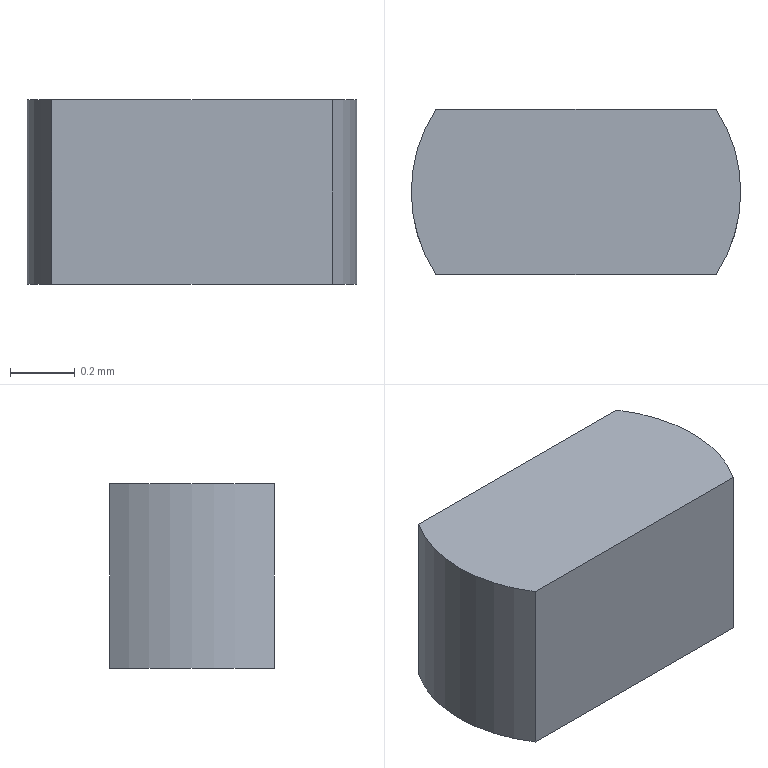Part | Creo | 1 solid | 6 faces | box 1.016 x 0.508 x 0.568 mm | volume 0.279 mm3 | plane 4 | cylinder 2 | commonest cylinder face diameters 0.923 x2
STEP:
#1=CARTESIAN_POINT('',(0.,0.,0.));
#2=DIRECTION('',(0.,0.,1.));
#3=DIRECTION('',(1.,0.,0.));
#4=AXIS2_PLACEMENT_3D('',#1,#2,#3);
#5=CARTESIAN_POINT('',(-0.4318,0.254,0.));
#6=VERTEX_POINT('',#5);
#7=CARTESIAN_POINT('',(-0.508,0.,0.));
#8=VERTEX_POINT('',#7);
#9=CARTESIAN_POINT('',(-0.04659,0.,0.));
#10=DIRECTION('',(0.,0.,1.));
#11=DIRECTION('',(-0.8348,0.5505,0.));
#12=AXIS2_PLACEMENT_3D('',#9,#10,#11);
#13=CIRCLE('',#12,0.4614);
#14=EDGE_CURVE('',#6,#8,#13,.T.);
#15=ORIENTED_EDGE('',*,*,#14,.T.);
#16=CARTESIAN_POINT('',(-0.4318,-0.254,0.));
#17=VERTEX_POINT('',#16);
#18=CARTESIAN_POINT('',(-0.04659,0.,0.));
#19=DIRECTION('',(0.,0.,1.));
#20=DIRECTION('',(-1.,0.,0.));
#21=AXIS2_PLACEMENT_3D('',#18,#19,#20);
#22=CIRCLE('',#21,0.4614);
#23=EDGE_CURVE('',#8,#17,#22,.T.);
#24=ORIENTED_EDGE('',*,*,#23,.T.);
#25=CARTESIAN_POINT('',(0.4318,-0.254,0.));
#26=VERTEX_POINT('',#25);
#27=CARTESIAN_POINT('',(-0.4318,-0.254,0.));
#28=DIRECTION('',(1.,0.,0.));
#29=VECTOR('',#28,0.8636);
#30=LINE('',#27,#29);
#31=EDGE_CURVE('',#17,#26,#30,.T.);
#32=ORIENTED_EDGE('',*,*,#31,.T.);
#33=CARTESIAN_POINT('',(0.508,0.,0.));
#34=VERTEX_POINT('',#33);
#35=CARTESIAN_POINT('',(0.04659,0.,0.));
#36=DIRECTION('',(0.,0.,1.));
#37=DIRECTION('',(0.8348,-0.5505,0.));
#38=AXIS2_PLACEMENT_3D('',#35,#36,#37);
#39=CIRCLE('',#38,0.4614);
#40=EDGE_CURVE('',#26,#34,#39,.T.);
#41=ORIENTED_EDGE('',*,*,#40,.T.);
#42=CARTESIAN_POINT('',(0.4318,0.254,0.));
#43=VERTEX_POINT('',#42);
#44=CARTESIAN_POINT('',(0.04659,0.,0.));
#45=DIRECTION('',(0.,0.,1.));
#46=DIRECTION('',(1.,0.,0.));
#47=AXIS2_PLACEMENT_3D('',#44,#45,#46);
#48=CIRCLE('',#47,0.4614);
#49=EDGE_CURVE('',#34,#43,#48,.T.);
#50=ORIENTED_EDGE('',*,*,#49,.T.);
#51=CARTESIAN_POINT('',(0.4318,0.254,0.));
#52=DIRECTION('',(-1.,0.,0.));
#53=VECTOR('',#52,0.8636);
#54=LINE('',#51,#53);
#55=EDGE_CURVE('',#43,#6,#54,.T.);
#56=ORIENTED_EDGE('',*,*,#55,.T.);
#57=EDGE_LOOP('',(#15,#24,#32,#41,#50,#56));
#58=FACE_OUTER_BOUND('',#57,.F.);
#59=CARTESIAN_POINT('',(0.,0.,0.));
#60=DIRECTION('',(0.,0.,1.));
#61=DIRECTION('',(1.,0.,0.));
#62=AXIS2_PLACEMENT_3D('',#59,#60,#61);
#63=PLANE('',#62);
#64=ADVANCED_FACE('',(#58),#63,.F.);
#65=ORIENTED_EDGE('',*,*,#23,.F.);
#66=ORIENTED_EDGE('',*,*,#14,.F.);
#67=CARTESIAN_POINT('',(-0.4318,0.254,0.568));
#68=VERTEX_POINT('',#67);
#69=CARTESIAN_POINT('',(-0.4318,0.254,0.));
#70=DIRECTION('',(0.,0.,1.));
#71=VECTOR('',#70,0.568);
#72=LINE('',#69,#71);
#73=EDGE_CURVE('',#6,#68,#72,.T.);
#74=ORIENTED_EDGE('',*,*,#73,.T.);
#75=CARTESIAN_POINT('',(-0.508,0.,0.568));
#76=VERTEX_POINT('',#75);
#77=CARTESIAN_POINT('',(-0.04659,0.,0.568));
#78=DIRECTION('',(0.,0.,-1.));
#79=DIRECTION('',(-1.,0.,0.));
#80=AXIS2_PLACEMENT_3D('',#77,#78,#79);
#81=CIRCLE('',#80,0.4614);
#82=EDGE_CURVE('',#76,#68,#81,.T.);
#83=ORIENTED_EDGE('',*,*,#82,.F.);
#84=CARTESIAN_POINT('',(-0.4318,-0.254,0.568));
#85=VERTEX_POINT('',#84);
#86=CARTESIAN_POINT('',(-0.04659,0.,0.568));
#87=DIRECTION('',(0.,0.,-1.));
#88=DIRECTION('',(-0.8348,-0.5505,0.));
#89=AXIS2_PLACEMENT_3D('',#86,#87,#88);
#90=CIRCLE('',#89,0.4614);
#91=EDGE_CURVE('',#85,#76,#90,.T.);
#92=ORIENTED_EDGE('',*,*,#91,.F.);
#93=CARTESIAN_POINT('',(-0.4318,-0.254,0.568));
#94=DIRECTION('',(0.,0.,-1.));
#95=VECTOR('',#94,0.568);
#96=LINE('',#93,#95);
#97=EDGE_CURVE('',#85,#17,#96,.T.);
#98=ORIENTED_EDGE('',*,*,#97,.T.);
#99=EDGE_LOOP('',(#65,#66,#74,#83,#92,#98));
#100=FACE_OUTER_BOUND('',#99,.F.);
#101=CARTESIAN_POINT('',(-0.04659,0.,0.));
#102=DIRECTION('',(0.,0.,1.));
#103=DIRECTION('',(1.,0.,0.));
#104=AXIS2_PLACEMENT_3D('',#101,#102,#103);
#105=CYLINDRICAL_SURFACE('',#104,0.4614);
#106=ADVANCED_FACE('',(#100),#105,.T.);
#107=ORIENTED_EDGE('',*,*,#55,.F.);
#108=CARTESIAN_POINT('',(0.4318,0.254,0.568));
#109=VERTEX_POINT('',#108);
#110=CARTESIAN_POINT('',(0.4318,0.254,0.568));
#111=DIRECTION('',(0.,0.,-1.));
#112=VECTOR('',#111,0.568);
#113=LINE('',#110,#112);
#114=EDGE_CURVE('',#109,#43,#113,.T.);
#115=ORIENTED_EDGE('',*,*,#114,.F.);
#116=CARTESIAN_POINT('',(0.4318,0.254,0.568));
#117=DIRECTION('',(-1.,0.,0.));
#118=VECTOR('',#117,0.8636);
#119=LINE('',#116,#118);
#120=EDGE_CURVE('',#109,#68,#119,.T.);
#121=ORIENTED_EDGE('',*,*,#120,.T.);
#122=ORIENTED_EDGE('',*,*,#73,.F.);
#123=EDGE_LOOP('',(#107,#115,#121,#122));
#124=FACE_OUTER_BOUND('',#123,.F.);
#125=CARTESIAN_POINT('',(0.4318,0.254,0.));
#126=DIRECTION('',(0.,1.,0.));
#127=DIRECTION('',(-1.,0.,0.));
#128=AXIS2_PLACEMENT_3D('',#125,#126,#127);
#129=PLANE('',#128);
#130=ADVANCED_FACE('',(#124),#129,.T.);
#131=ORIENTED_EDGE('',*,*,#49,.F.);
#132=ORIENTED_EDGE('',*,*,#40,.F.);
#133=CARTESIAN_POINT('',(0.4318,-0.254,0.568));
#134=VERTEX_POINT('',#133);
#135=CARTESIAN_POINT('',(0.4318,-0.254,0.));
#136=DIRECTION('',(0.,0.,1.));
#137=VECTOR('',#136,0.568);
#138=LINE('',#135,#137);
#139=EDGE_CURVE('',#26,#134,#138,.T.);
#140=ORIENTED_EDGE('',*,*,#139,.T.);
#141=CARTESIAN_POINT('',(0.508,0.,0.568));
#142=VERTEX_POINT('',#141);
#143=CARTESIAN_POINT('',(0.04659,0.,0.568));
#144=DIRECTION('',(0.,0.,-1.));
#145=DIRECTION('',(1.,0.,0.));
#146=AXIS2_PLACEMENT_3D('',#143,#144,#145);
#147=CIRCLE('',#146,0.4614);
#148=EDGE_CURVE('',#142,#134,#147,.T.);
#149=ORIENTED_EDGE('',*,*,#148,.F.);
#150=CARTESIAN_POINT('',(0.04659,0.,0.568));
#151=DIRECTION('',(0.,0.,-1.));
#152=DIRECTION('',(0.8348,0.5505,0.));
#153=AXIS2_PLACEMENT_3D('',#150,#151,#152);
#154=CIRCLE('',#153,0.4614);
#155=EDGE_CURVE('',#109,#142,#154,.T.);
#156=ORIENTED_EDGE('',*,*,#155,.F.);
#157=ORIENTED_EDGE('',*,*,#114,.T.);
#158=EDGE_LOOP('',(#131,#132,#140,#149,#156,#157));
#159=FACE_OUTER_BOUND('',#158,.F.);
#160=CARTESIAN_POINT('',(0.04659,0.,0.));
#161=DIRECTION('',(0.,0.,1.));
#162=DIRECTION('',(1.,0.,0.));
#163=AXIS2_PLACEMENT_3D('',#160,#161,#162);
#164=CYLINDRICAL_SURFACE('',#163,0.4614);
#165=ADVANCED_FACE('',(#159),#164,.T.);
#166=ORIENTED_EDGE('',*,*,#31,.F.);
#167=ORIENTED_EDGE('',*,*,#97,.F.);
#168=CARTESIAN_POINT('',(-0.4318,-0.254,0.568));
#169=DIRECTION('',(1.,0.,0.));
#170=VECTOR('',#169,0.8636);
#171=LINE('',#168,#170);
#172=EDGE_CURVE('',#85,#134,#171,.T.);
#173=ORIENTED_EDGE('',*,*,#172,.T.);
#174=ORIENTED_EDGE('',*,*,#139,.F.);
#175=EDGE_LOOP('',(#166,#167,#173,#174));
#176=FACE_OUTER_BOUND('',#175,.F.);
#177=CARTESIAN_POINT('',(-0.4318,-0.254,0.));
#178=DIRECTION('',(0.,-1.,0.));
#179=DIRECTION('',(1.,0.,0.));
#180=AXIS2_PLACEMENT_3D('',#177,#178,#179);
#181=PLANE('',#180);
#182=ADVANCED_FACE('',(#176),#181,.T.);
#183=ORIENTED_EDGE('',*,*,#91,.T.);
#184=ORIENTED_EDGE('',*,*,#82,.T.);
#185=ORIENTED_EDGE('',*,*,#120,.F.);
#186=ORIENTED_EDGE('',*,*,#155,.T.);
#187=ORIENTED_EDGE('',*,*,#148,.T.);
#188=ORIENTED_EDGE('',*,*,#172,.F.);
#189=EDGE_LOOP('',(#183,#184,#185,#186,#187,#188));
#190=FACE_OUTER_BOUND('',#189,.F.);
#191=CARTESIAN_POINT('',(0.,0.,0.568));
#192=DIRECTION('',(0.,0.,1.));
#193=DIRECTION('',(1.,0.,0.));
#194=AXIS2_PLACEMENT_3D('',#191,#192,#193);
#195=PLANE('',#194);
#196=ADVANCED_FACE('',(#190),#195,.T.);
#197=CLOSED_SHELL('',(#64,#106,#130,#165,#182,#196));
#198=MANIFOLD_SOLID_BREP('',#197);
#199=(LENGTH_UNIT()NAMED_UNIT(*)SI_UNIT(.MILLI.,.METRE.));
#200=UNCERTAINTY_MEASURE_WITH_UNIT(LENGTH_MEASURE(0.000127),#199,'','');
#201=(NAMED_UNIT(*)PLANE_ANGLE_UNIT()SI_UNIT($,.RADIAN.));
#202=PLANE_ANGLE_MEASURE_WITH_UNIT(PLANE_ANGLE_MEASURE(0.01745),#201);
#203=(CONVERSION_BASED_UNIT('DEGREE',#202)NAMED_UNIT(*)PLANE_ANGLE_UNIT());
#204=(NAMED_UNIT(*)SI_UNIT($,.STERADIAN.)SOLID_ANGLE_UNIT());
#205=(GEOMETRIC_REPRESENTATION_CONTEXT(3)GLOBAL_UNCERTAINTY_ASSIGNED_CONTEXT((#200))GLOBAL_UNIT_ASSIGNED_CONTEXT((#199,#203,#204))REPRESENTATION_CONTEXT('',''));
#206=ADVANCED_BREP_SHAPE_REPRESENTATION('',(#4,#198),#205);